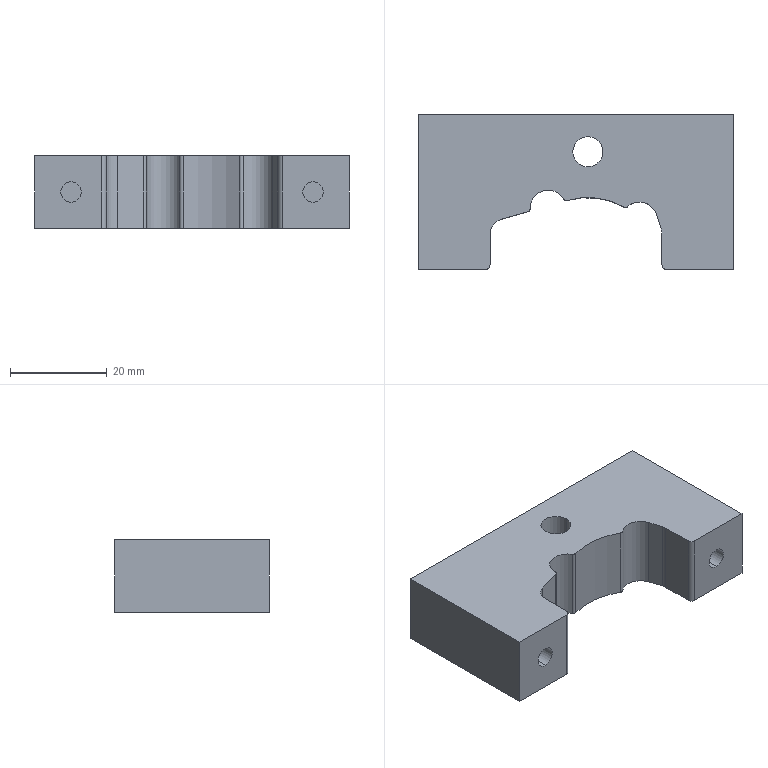Part | 1 solid | 30 faces | volume 23198 mm3 | cylinder 17 | plane 13 | commonest cylinder face diameters 4.2 x4 1.4 x3 7.4 x3 2 x2 6.2 x2 6 x1